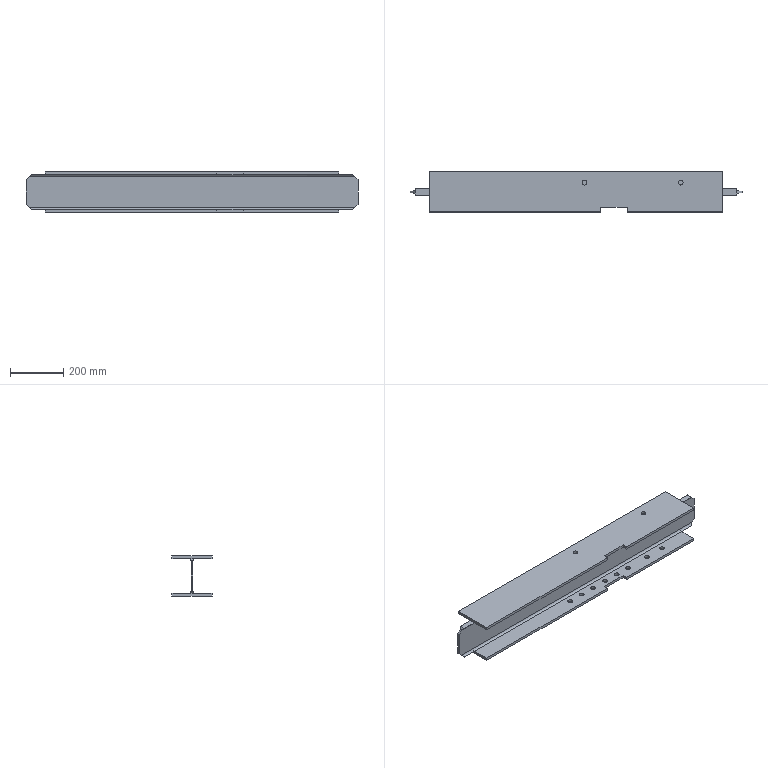Part | STEP file | 02-Longitudinal beam H150X150_default<machining> | 1 solid | 74 faces | box 1243 x 150 x 150 mm | volume 4402012 mm3 | cylinder 40 | plane 34 | commonest cylinder face diameters 18 x36 16 x4